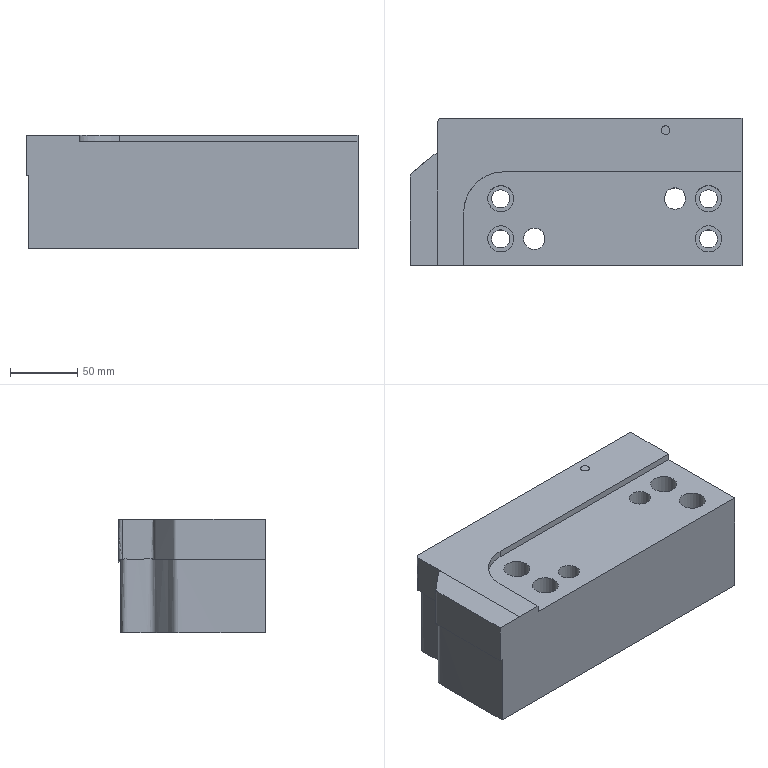Part | NX | features solid 2 | 1 solid | 29 faces | box 247.727 x 110 x 85 mm | volume 2013401 mm3 | cylinder 11 | plane 11 | spline 7 | commonest cylinder face diameters 13.5 x4 19.5 x4 16 x2 60 x1